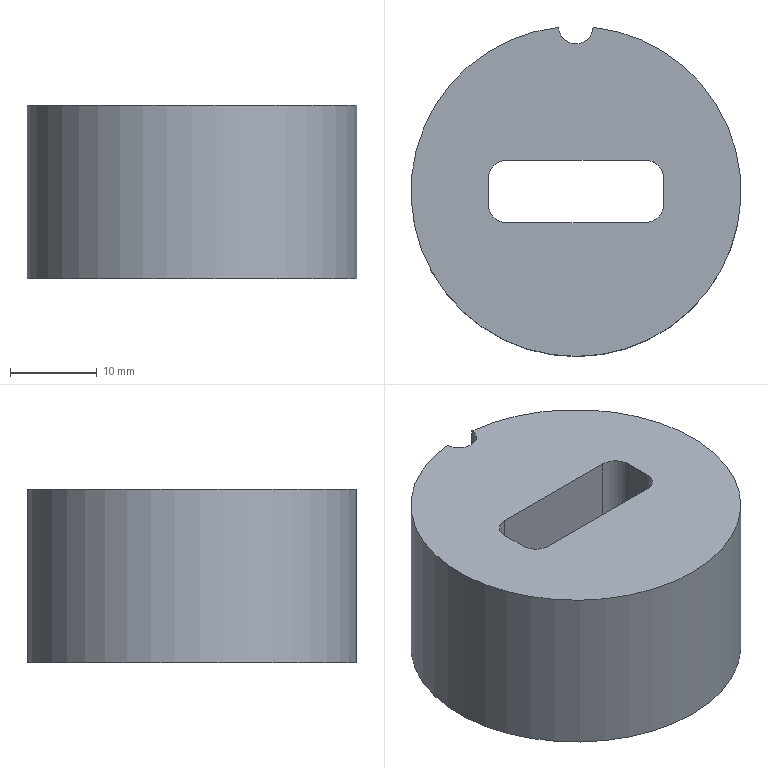Part | NX | features solid 2 | 1 solid | 14 faces | box 38 x 37.897 x 20 mm | volume 14764 mm3 | plane 7 | cylinder 7 | commonest cylinder face diameters 4.17 x4 4 x1 26.6 x1 38 x1
STEP:
#1=CARTESIAN_POINT('',(-663.326,-80.935,26.875));
#2=VERTEX_POINT('',#1);
#3=CARTESIAN_POINT('',(-667.321,-80.939,26.875));
#4=VERTEX_POINT('',#3);
#5=CARTESIAN_POINT('',(-665.324,-80.831,26.875));
#6=DIRECTION('',(0.,0.,-1.));
#7=DIRECTION('',(0.001034,-1.,0.));
#8=AXIS2_PLACEMENT_3D('',#5,#6,#7);
#9=CIRCLE('',#8,2.);
#10=EDGE_CURVE('',#2,#4,#9,.T.);
#11=ORIENTED_EDGE('',*,*,#10,.T.);
#12=CARTESIAN_POINT('',(-665.304,-99.831,26.875));
#13=DIRECTION('',(0.,0.,-1.));
#14=DIRECTION('',(0.001034,-1.,0.));
#15=AXIS2_PLACEMENT_3D('',#12,#13,#14);
#16=CIRCLE('',#15,19.);
#17=EDGE_CURVE('',#2,#4,#16,.T.);
#18=ORIENTED_EDGE('',*,*,#17,.F.);
#19=EDGE_LOOP('',(#11,#18));
#20=FACE_BOUND('',#19,.T.);
#21=CARTESIAN_POINT('',(-673.308,-96.255,26.875));
#22=VERTEX_POINT('',#21);
#23=CARTESIAN_POINT('',(-675.39,-98.342,26.875));
#24=VERTEX_POINT('',#23);
#25=CARTESIAN_POINT('',(-673.305,-98.34,26.875));
#26=DIRECTION('',(0.,0.,1.));
#27=DIRECTION('',(-1.,0.,0.));
#28=AXIS2_PLACEMENT_3D('',#25,#26,#27);
#29=CIRCLE('',#28,2.085);
#30=EDGE_CURVE('',#22,#24,#29,.T.);
#31=ORIENTED_EDGE('',*,*,#30,.F.);
#32=CARTESIAN_POINT('',(-657.308,-96.238,26.875));
#33=VERTEX_POINT('',#32);
#34=CARTESIAN_POINT('',(-665.308,-96.246,26.875));
#35=DIRECTION('',(1.,0.001034,0.));
#36=VECTOR('',#35,1000.);
#37=LINE('',#34,#36);
#38=EDGE_CURVE('',#22,#33,#37,.T.);
#39=ORIENTED_EDGE('',*,*,#38,.T.);
#40=CARTESIAN_POINT('',(-655.22,-98.321,26.875));
#41=VERTEX_POINT('',#40);
#42=CARTESIAN_POINT('',(-657.305,-98.323,26.875));
#43=DIRECTION('',(0.,0.,1.));
#44=DIRECTION('',(-1.,0.,0.));
#45=AXIS2_PLACEMENT_3D('',#42,#43,#44);
#46=CIRCLE('',#45,2.085);
#47=EDGE_CURVE('',#41,#33,#46,.T.);
#48=ORIENTED_EDGE('',*,*,#47,.F.);
#49=CARTESIAN_POINT('',(-655.217,-101.321,26.875));
#50=VERTEX_POINT('',#49);
#51=CARTESIAN_POINT('',(-655.219,-99.821,26.875));
#52=DIRECTION('',(0.001034,-1.,0.));
#53=VECTOR('',#52,1000.);
#54=LINE('',#51,#53);
#55=EDGE_CURVE('',#41,#50,#54,.T.);
#56=ORIENTED_EDGE('',*,*,#55,.T.);
#57=CARTESIAN_POINT('',(-657.3,-103.408,26.875));
#58=VERTEX_POINT('',#57);
#59=CARTESIAN_POINT('',(-657.302,-101.323,26.875));
#60=DIRECTION('',(0.,0.,1.));
#61=DIRECTION('',(-1.,0.,0.));
#62=AXIS2_PLACEMENT_3D('',#59,#60,#61);
#63=CIRCLE('',#62,2.085);
#64=EDGE_CURVE('',#58,#50,#63,.T.);
#65=ORIENTED_EDGE('',*,*,#64,.F.);
#66=CARTESIAN_POINT('',(-673.3,-103.425,26.875));
#67=VERTEX_POINT('',#66);
#68=CARTESIAN_POINT('',(-665.3,-103.416,26.875));
#69=DIRECTION('',(-1.,-0.001034,0.));
#70=VECTOR('',#69,1000.);
#71=LINE('',#68,#70);
#72=EDGE_CURVE('',#58,#67,#71,.T.);
#73=ORIENTED_EDGE('',*,*,#72,.T.);
#74=CARTESIAN_POINT('',(-675.387,-101.342,26.875));
#75=VERTEX_POINT('',#74);
#76=CARTESIAN_POINT('',(-673.302,-101.34,26.875));
#77=DIRECTION('',(0.,0.,1.));
#78=DIRECTION('',(-1.,0.,0.));
#79=AXIS2_PLACEMENT_3D('',#76,#77,#78);
#80=CIRCLE('',#79,2.085);
#81=EDGE_CURVE('',#75,#67,#80,.T.);
#82=ORIENTED_EDGE('',*,*,#81,.F.);
#83=CARTESIAN_POINT('',(-675.389,-99.842,26.875));
#84=DIRECTION('',(-0.001034,1.,0.));
#85=VECTOR('',#84,1000.);
#86=LINE('',#83,#85);
#87=EDGE_CURVE('',#75,#24,#86,.T.);
#88=ORIENTED_EDGE('',*,*,#87,.T.);
#89=EDGE_LOOP('',(#31,#39,#48,#56,#65,#73,#82,#88));
#90=FACE_BOUND('',#89,.T.);
#91=CARTESIAN_POINT('',(-665.304,-99.831,26.875));
#92=DIRECTION('',(0.,0.,1.));
#93=DIRECTION('',(-0.001034,1.,0.));
#94=AXIS2_PLACEMENT_3D('',#91,#92,#93);
#95=PLANE('',#94);
#96=ADVANCED_FACE('',(#20,#90),#95,.T.);
#97=CARTESIAN_POINT('',(-667.321,-80.939,6.875));
#98=VERTEX_POINT('',#97);
#99=CARTESIAN_POINT('',(-663.326,-80.935,6.875));
#100=VERTEX_POINT('',#99);
#101=CARTESIAN_POINT('',(-665.324,-80.831,6.875));
#102=DIRECTION('',(0.,0.,1.));
#103=DIRECTION('',(-0.001034,1.,0.));
#104=AXIS2_PLACEMENT_3D('',#101,#102,#103);
#105=CIRCLE('',#104,2.);
#106=EDGE_CURVE('',#98,#100,#105,.T.);
#107=ORIENTED_EDGE('',*,*,#106,.T.);
#108=CARTESIAN_POINT('',(-665.304,-99.831,6.875));
#109=DIRECTION('',(0.,0.,1.));
#110=DIRECTION('',(-0.001034,1.,0.));
#111=AXIS2_PLACEMENT_3D('',#108,#109,#110);
#112=CIRCLE('',#111,19.);
#113=EDGE_CURVE('',#98,#100,#112,.T.);
#114=ORIENTED_EDGE('',*,*,#113,.F.);
#115=EDGE_LOOP('',(#107,#114));
#116=FACE_BOUND('',#115,.T.);
#117=CARTESIAN_POINT('',(-665.318,-86.531,6.875));
#118=VERTEX_POINT('',#117);
#119=CARTESIAN_POINT('',(-665.304,-99.831,6.875));
#120=DIRECTION('',(0.,0.,1.));
#121=DIRECTION('',(-0.001034,1.,0.));
#122=AXIS2_PLACEMENT_3D('',#119,#120,#121);
#123=CIRCLE('',#122,13.3);
#124=EDGE_CURVE('',#118,#118,#123,.T.);
#125=ORIENTED_EDGE('',*,*,#124,.T.);
#126=EDGE_LOOP('',(#125));
#127=FACE_BOUND('',#126,.T.);
#128=CARTESIAN_POINT('',(-665.304,-99.831,6.875));
#129=DIRECTION('',(0.,0.,-1.));
#130=DIRECTION('',(0.001034,-1.,0.));
#131=AXIS2_PLACEMENT_3D('',#128,#129,#130);
#132=PLANE('',#131);
#133=ADVANCED_FACE('',(#116,#127),#132,.T.);
#134=CARTESIAN_POINT('',(-667.321,-80.939,16.875));
#135=DIRECTION('',(0.,0.,1.));
#136=VECTOR('',#135,1000.);
#137=LINE('',#134,#136);
#138=EDGE_CURVE('',#98,#4,#137,.T.);
#139=ORIENTED_EDGE('',*,*,#138,.F.);
#140=ORIENTED_EDGE('',*,*,#113,.T.);
#141=CARTESIAN_POINT('',(-663.326,-80.935,16.875));
#142=DIRECTION('',(0.,0.,1.));
#143=VECTOR('',#142,1000.);
#144=LINE('',#141,#143);
#145=EDGE_CURVE('',#2,#100,#144,.F.);
#146=ORIENTED_EDGE('',*,*,#145,.F.);
#147=ORIENTED_EDGE('',*,*,#17,.T.);
#148=EDGE_LOOP('',(#139,#140,#146,#147));
#149=FACE_BOUND('',#148,.T.);
#150=CARTESIAN_POINT('',(-665.304,-99.831,6.875));
#151=DIRECTION('',(0.,0.,1.));
#152=DIRECTION('',(-0.001034,1.,0.));
#153=AXIS2_PLACEMENT_3D('',#150,#151,#152);
#154=CYLINDRICAL_SURFACE('',#153,19.);
#155=ADVANCED_FACE('',(#149),#154,.T.);
#156=CARTESIAN_POINT('',(-657.308,-96.238,18.875));
#157=VERTEX_POINT('',#156);
#158=CARTESIAN_POINT('',(-673.308,-96.255,18.875));
#159=VERTEX_POINT('',#158);
#160=CARTESIAN_POINT('',(-665.308,-96.246,18.875));
#161=DIRECTION('',(-1.,-0.001034,0.));
#162=VECTOR('',#161,1000.);
#163=LINE('',#160,#162);
#164=EDGE_CURVE('',#157,#159,#163,.T.);
#165=ORIENTED_EDGE('',*,*,#164,.T.);
#166=CARTESIAN_POINT('',(-675.39,-98.342,18.875));
#167=VERTEX_POINT('',#166);
#168=CARTESIAN_POINT('',(-673.305,-98.34,18.875));
#169=DIRECTION('',(0.,0.,-1.));
#170=DIRECTION('',(1.,0.,0.));
#171=AXIS2_PLACEMENT_3D('',#168,#169,#170);
#172=CIRCLE('',#171,2.085);
#173=EDGE_CURVE('',#167,#159,#172,.T.);
#174=ORIENTED_EDGE('',*,*,#173,.F.);
#175=CARTESIAN_POINT('',(-675.387,-101.342,18.875));
#176=VERTEX_POINT('',#175);
#177=CARTESIAN_POINT('',(-675.389,-99.842,18.875));
#178=DIRECTION('',(0.001034,-1.,0.));
#179=VECTOR('',#178,1000.);
#180=LINE('',#177,#179);
#181=EDGE_CURVE('',#167,#176,#180,.T.);
#182=ORIENTED_EDGE('',*,*,#181,.T.);
#183=CARTESIAN_POINT('',(-673.3,-103.425,18.875));
#184=VERTEX_POINT('',#183);
#185=CARTESIAN_POINT('',(-673.302,-101.34,18.875));
#186=DIRECTION('',(0.,0.,-1.));
#187=DIRECTION('',(1.,0.,0.));
#188=AXIS2_PLACEMENT_3D('',#185,#186,#187);
#189=CIRCLE('',#188,2.085);
#190=EDGE_CURVE('',#184,#176,#189,.T.);
#191=ORIENTED_EDGE('',*,*,#190,.F.);
#192=CARTESIAN_POINT('',(-657.3,-103.408,18.875));
#193=VERTEX_POINT('',#192);
#194=CARTESIAN_POINT('',(-665.3,-103.416,18.875));
#195=DIRECTION('',(1.,0.001034,0.));
#196=VECTOR('',#195,1000.);
#197=LINE('',#194,#196);
#198=EDGE_CURVE('',#184,#193,#197,.T.);
#199=ORIENTED_EDGE('',*,*,#198,.T.);
#200=CARTESIAN_POINT('',(-655.217,-101.321,18.875));
#201=VERTEX_POINT('',#200);
#202=CARTESIAN_POINT('',(-657.302,-101.323,18.875));
#203=DIRECTION('',(0.,0.,-1.));
#204=DIRECTION('',(1.,0.,0.));
#205=AXIS2_PLACEMENT_3D('',#202,#203,#204);
#206=CIRCLE('',#205,2.085);
#207=EDGE_CURVE('',#201,#193,#206,.T.);
#208=ORIENTED_EDGE('',*,*,#207,.F.);
#209=CARTESIAN_POINT('',(-655.22,-98.321,18.875));
#210=VERTEX_POINT('',#209);
#211=CARTESIAN_POINT('',(-655.219,-99.821,18.875));
#212=DIRECTION('',(-0.001034,1.,0.));
#213=VECTOR('',#212,1000.);
#214=LINE('',#211,#213);
#215=EDGE_CURVE('',#201,#210,#214,.T.);
#216=ORIENTED_EDGE('',*,*,#215,.T.);
#217=CARTESIAN_POINT('',(-657.305,-98.323,18.875));
#218=DIRECTION('',(0.,0.,-1.));
#219=DIRECTION('',(1.,0.,0.));
#220=AXIS2_PLACEMENT_3D('',#217,#218,#219);
#221=CIRCLE('',#220,2.085);
#222=EDGE_CURVE('',#157,#210,#221,.T.);
#223=ORIENTED_EDGE('',*,*,#222,.F.);
#224=EDGE_LOOP('',(#165,#174,#182,#191,#199,#208,#216,#223));
#225=FACE_BOUND('',#224,.T.);
#226=CARTESIAN_POINT('',(-665.29,-113.131,18.875));
#227=VERTEX_POINT('',#226);
#228=CARTESIAN_POINT('',(-665.304,-99.831,18.875));
#229=DIRECTION('',(0.,0.,-1.));
#230=DIRECTION('',(0.001034,-1.,0.));
#231=AXIS2_PLACEMENT_3D('',#228,#229,#230);
#232=CIRCLE('',#231,13.3);
#233=EDGE_CURVE('',#227,#227,#232,.T.);
#234=ORIENTED_EDGE('',*,*,#233,.T.);
#235=EDGE_LOOP('',(#234));
#236=FACE_BOUND('',#235,.T.);
#237=CARTESIAN_POINT('',(-665.304,-99.831,18.875));
#238=DIRECTION('',(0.,0.,1.));
#239=DIRECTION('',(-0.001034,1.,0.));
#240=AXIS2_PLACEMENT_3D('',#237,#238,#239);
#241=PLANE('',#240);
#242=ADVANCED_FACE('',(#225,#236),#241,.F.);
#243=ORIENTED_EDGE('',*,*,#233,.F.);
#244=EDGE_LOOP('',(#243));
#245=FACE_BOUND('',#244,.T.);
#246=ORIENTED_EDGE('',*,*,#124,.F.);
#247=EDGE_LOOP('',(#246));
#248=FACE_BOUND('',#247,.T.);
#249=CARTESIAN_POINT('',(-665.304,-99.831,6.875));
#250=DIRECTION('',(0.,0.,1.));
#251=DIRECTION('',(-0.001034,1.,0.));
#252=AXIS2_PLACEMENT_3D('',#249,#250,#251);
#253=CYLINDRICAL_SURFACE('',#252,13.3);
#254=ADVANCED_FACE('',(#245,#248),#253,.F.);
#255=ORIENTED_EDGE('',*,*,#215,.F.);
#256=CARTESIAN_POINT('',(-655.217,-101.321,18.875));
#257=DIRECTION('',(0.,0.,1.));
#258=VECTOR('',#257,1000.);
#259=LINE('',#256,#258);
#260=EDGE_CURVE('',#50,#201,#259,.F.);
#261=ORIENTED_EDGE('',*,*,#260,.F.);
#262=ORIENTED_EDGE('',*,*,#55,.F.);
#263=CARTESIAN_POINT('',(-655.22,-98.321,18.875));
#264=DIRECTION('',(0.,0.,1.));
#265=VECTOR('',#264,1000.);
#266=LINE('',#263,#265);
#267=EDGE_CURVE('',#210,#41,#266,.T.);
#268=ORIENTED_EDGE('',*,*,#267,.F.);
#269=EDGE_LOOP('',(#255,#261,#262,#268));
#270=FACE_BOUND('',#269,.T.);
#271=CARTESIAN_POINT('',(-655.219,-99.821,18.875));
#272=DIRECTION('',(1.,0.001034,0.));
#273=DIRECTION('',(0.,0.,-1.));
#274=AXIS2_PLACEMENT_3D('',#271,#272,#273);
#275=PLANE('',#274);
#276=ADVANCED_FACE('',(#270),#275,.F.);
#277=ORIENTED_EDGE('',*,*,#72,.F.);
#278=CARTESIAN_POINT('',(-657.3,-103.408,18.875));
#279=DIRECTION('',(0.,0.,1.));
#280=VECTOR('',#279,1000.);
#281=LINE('',#278,#280);
#282=EDGE_CURVE('',#193,#58,#281,.T.);
#283=ORIENTED_EDGE('',*,*,#282,.F.);
#284=ORIENTED_EDGE('',*,*,#198,.F.);
#285=CARTESIAN_POINT('',(-673.3,-103.425,18.875));
#286=DIRECTION('',(0.,0.,1.));
#287=VECTOR('',#286,1000.);
#288=LINE('',#285,#287);
#289=EDGE_CURVE('',#67,#184,#288,.F.);
#290=ORIENTED_EDGE('',*,*,#289,.F.);
#291=EDGE_LOOP('',(#277,#283,#284,#290));
#292=FACE_BOUND('',#291,.T.);
#293=CARTESIAN_POINT('',(-665.3,-103.416,18.875));
#294=DIRECTION('',(0.001034,-1.,0.));
#295=DIRECTION('',(0.,0.,1.));
#296=AXIS2_PLACEMENT_3D('',#293,#294,#295);
#297=PLANE('',#296);
#298=ADVANCED_FACE('',(#292),#297,.F.);
#299=ORIENTED_EDGE('',*,*,#87,.F.);
#300=CARTESIAN_POINT('',(-675.387,-101.342,18.875));
#301=DIRECTION('',(0.,0.,1.));
#302=VECTOR('',#301,1000.);
#303=LINE('',#300,#302);
#304=EDGE_CURVE('',#176,#75,#303,.T.);
#305=ORIENTED_EDGE('',*,*,#304,.F.);
#306=ORIENTED_EDGE('',*,*,#181,.F.);
#307=CARTESIAN_POINT('',(-675.39,-98.342,18.875));
#308=DIRECTION('',(0.,0.,1.));
#309=VECTOR('',#308,1000.);
#310=LINE('',#307,#309);
#311=EDGE_CURVE('',#24,#167,#310,.F.);
#312=ORIENTED_EDGE('',*,*,#311,.F.);
#313=EDGE_LOOP('',(#299,#305,#306,#312));
#314=FACE_BOUND('',#313,.T.);
#315=CARTESIAN_POINT('',(-675.389,-99.842,18.875));
#316=DIRECTION('',(-1.,-0.001034,0.));
#317=DIRECTION('',(0.,0.,1.));
#318=AXIS2_PLACEMENT_3D('',#315,#316,#317);
#319=PLANE('',#318);
#320=ADVANCED_FACE('',(#314),#319,.F.);
#321=ORIENTED_EDGE('',*,*,#38,.F.);
#322=CARTESIAN_POINT('',(-673.308,-96.255,18.875));
#323=DIRECTION('',(0.,0.,1.));
#324=VECTOR('',#323,1000.);
#325=LINE('',#322,#324);
#326=EDGE_CURVE('',#159,#22,#325,.T.);
#327=ORIENTED_EDGE('',*,*,#326,.F.);
#328=ORIENTED_EDGE('',*,*,#164,.F.);
#329=CARTESIAN_POINT('',(-657.308,-96.238,18.875));
#330=DIRECTION('',(0.,0.,1.));
#331=VECTOR('',#330,1000.);
#332=LINE('',#329,#331);
#333=EDGE_CURVE('',#33,#157,#332,.F.);
#334=ORIENTED_EDGE('',*,*,#333,.F.);
#335=EDGE_LOOP('',(#321,#327,#328,#334));
#336=FACE_BOUND('',#335,.T.);
#337=CARTESIAN_POINT('',(-665.308,-96.246,18.875));
#338=DIRECTION('',(-0.001034,1.,0.));
#339=DIRECTION('',(0.,0.,-1.));
#340=AXIS2_PLACEMENT_3D('',#337,#338,#339);
#341=PLANE('',#340);
#342=ADVANCED_FACE('',(#336),#341,.F.);
#343=ORIENTED_EDGE('',*,*,#222,.T.);
#344=ORIENTED_EDGE('',*,*,#267,.T.);
#345=ORIENTED_EDGE('',*,*,#47,.T.);
#346=ORIENTED_EDGE('',*,*,#333,.T.);
#347=EDGE_LOOP('',(#343,#344,#345,#346));
#348=FACE_BOUND('',#347,.T.);
#349=CARTESIAN_POINT('',(-657.305,-98.323,18.875));
#350=DIRECTION('',(0.,0.,1.));
#351=DIRECTION('',(-1.,0.,0.));
#352=AXIS2_PLACEMENT_3D('',#349,#350,#351);
#353=CYLINDRICAL_SURFACE('',#352,2.085);
#354=ADVANCED_FACE('',(#348),#353,.F.);
#355=ORIENTED_EDGE('',*,*,#173,.T.);
#356=ORIENTED_EDGE('',*,*,#326,.T.);
#357=ORIENTED_EDGE('',*,*,#30,.T.);
#358=ORIENTED_EDGE('',*,*,#311,.T.);
#359=EDGE_LOOP('',(#355,#356,#357,#358));
#360=FACE_BOUND('',#359,.T.);
#361=CARTESIAN_POINT('',(-673.305,-98.34,18.875));
#362=DIRECTION('',(0.,0.,1.));
#363=DIRECTION('',(-1.,0.,0.));
#364=AXIS2_PLACEMENT_3D('',#361,#362,#363);
#365=CYLINDRICAL_SURFACE('',#364,2.085);
#366=ADVANCED_FACE('',(#360),#365,.F.);
#367=ORIENTED_EDGE('',*,*,#190,.T.);
#368=ORIENTED_EDGE('',*,*,#304,.T.);
#369=ORIENTED_EDGE('',*,*,#81,.T.);
#370=ORIENTED_EDGE('',*,*,#289,.T.);
#371=EDGE_LOOP('',(#367,#368,#369,#370));
#372=FACE_BOUND('',#371,.T.);
#373=CARTESIAN_POINT('',(-673.302,-101.34,18.875));
#374=DIRECTION('',(0.,0.,1.));
#375=DIRECTION('',(-1.,0.,0.));
#376=AXIS2_PLACEMENT_3D('',#373,#374,#375);
#377=CYLINDRICAL_SURFACE('',#376,2.085);
#378=ADVANCED_FACE('',(#372),#377,.F.);
#379=ORIENTED_EDGE('',*,*,#207,.T.);
#380=ORIENTED_EDGE('',*,*,#282,.T.);
#381=ORIENTED_EDGE('',*,*,#64,.T.);
#382=ORIENTED_EDGE('',*,*,#260,.T.);
#383=EDGE_LOOP('',(#379,#380,#381,#382));
#384=FACE_BOUND('',#383,.T.);
#385=CARTESIAN_POINT('',(-657.302,-101.323,18.875));
#386=DIRECTION('',(0.,0.,1.));
#387=DIRECTION('',(-1.,0.,0.));
#388=AXIS2_PLACEMENT_3D('',#385,#386,#387);
#389=CYLINDRICAL_SURFACE('',#388,2.085);
#390=ADVANCED_FACE('',(#384),#389,.F.);
#391=ORIENTED_EDGE('',*,*,#138,.T.);
#392=ORIENTED_EDGE('',*,*,#10,.F.);
#393=ORIENTED_EDGE('',*,*,#145,.T.);
#394=ORIENTED_EDGE('',*,*,#106,.F.);
#395=EDGE_LOOP('',(#391,#392,#393,#394));
#396=FACE_BOUND('',#395,.T.);
#397=CARTESIAN_POINT('',(-665.324,-80.831,6.875));
#398=DIRECTION('',(0.,0.,1.));
#399=DIRECTION('',(-0.001034,1.,0.));
#400=AXIS2_PLACEMENT_3D('',#397,#398,#399);
#401=CYLINDRICAL_SURFACE('',#400,2.);
#402=ADVANCED_FACE('',(#396),#401,.F.);
#403=CLOSED_SHELL('',(#96,#133,#155,#242,#254,#276,#298,#320,#342,#354,#366,#378,#390,#402));
#404=MANIFOLD_SOLID_BREP('',#403);
#405=(LENGTH_UNIT()NAMED_UNIT(*)SI_UNIT(.MILLI.,.METRE.));
#406=UNCERTAINTY_MEASURE_WITH_UNIT(LENGTH_MEASURE(0.00001),#405,'','');
#407=(NAMED_UNIT(*)PLANE_ANGLE_UNIT()SI_UNIT($,.RADIAN.));
#408=(NAMED_UNIT(*)SI_UNIT($,.STERADIAN.)SOLID_ANGLE_UNIT());
#409=(GEOMETRIC_REPRESENTATION_CONTEXT(3)GLOBAL_UNCERTAINTY_ASSIGNED_CONTEXT((#406))GLOBAL_UNIT_ASSIGNED_CONTEXT((#405,#407,#408))REPRESENTATION_CONTEXT('',''));
#410=ADVANCED_BREP_SHAPE_REPRESENTATION('',(#404),#409);